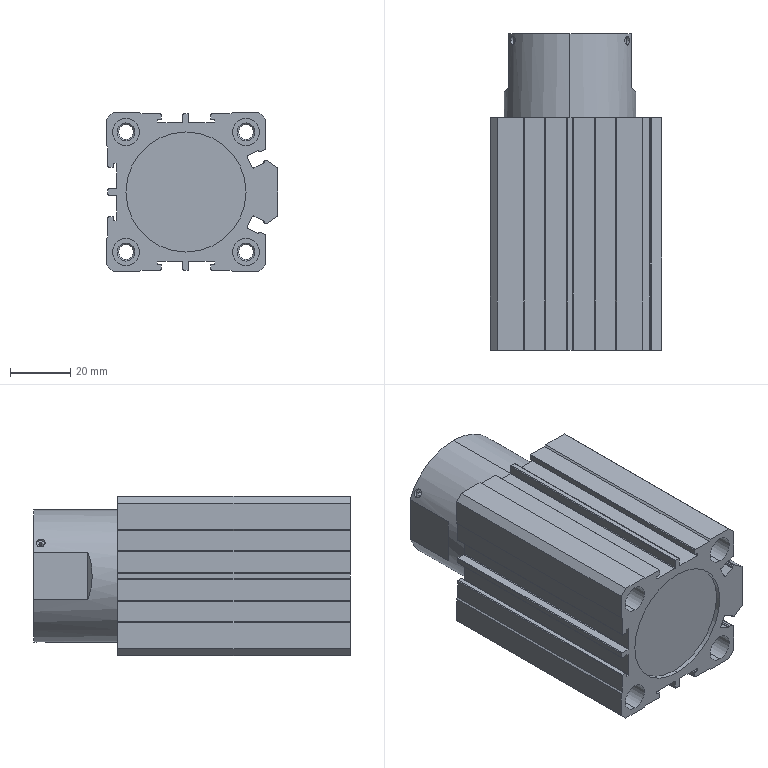Part | SolidWorks | features BaseBody 1 | 1 solid | 229 faces | box 57 x 105.5 x 53 mm | volume 155385 mm3 | plane 104 | cylinder 101 | cone 24 | commonest cylinder face diameters 0.4 x41 9 x16 0.8 x10 4.917 x8 3 x6 1 x5